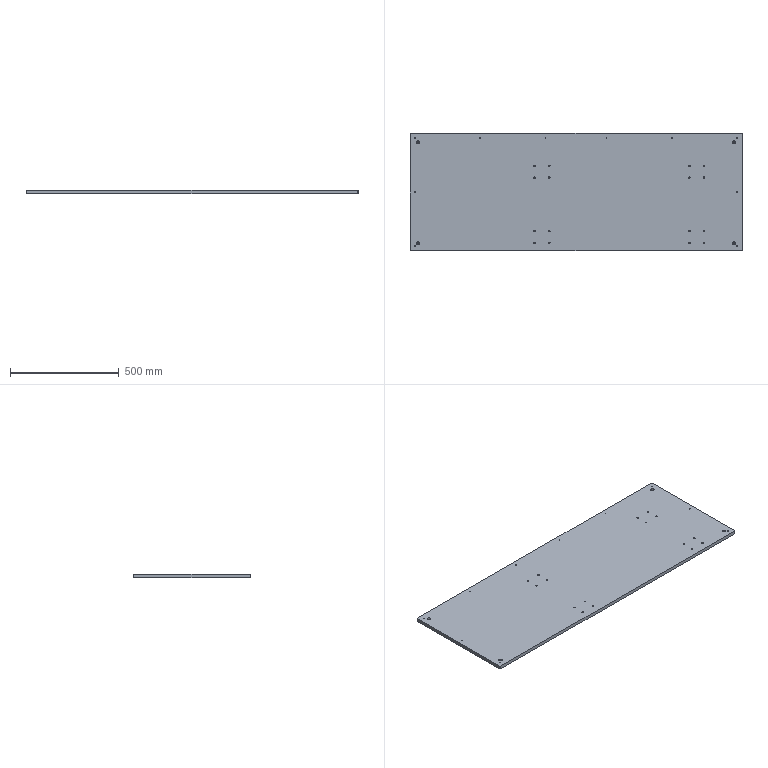Part | NX | features BREP 1 | 1 solid | 82 faces | box 1526 x 541 x 16 mm | volume 13189631 mm3 | cylinder 68 | plane 14 | commonest cylinder face diameters 7 x32 3.3 x20 9 x8 15 x8